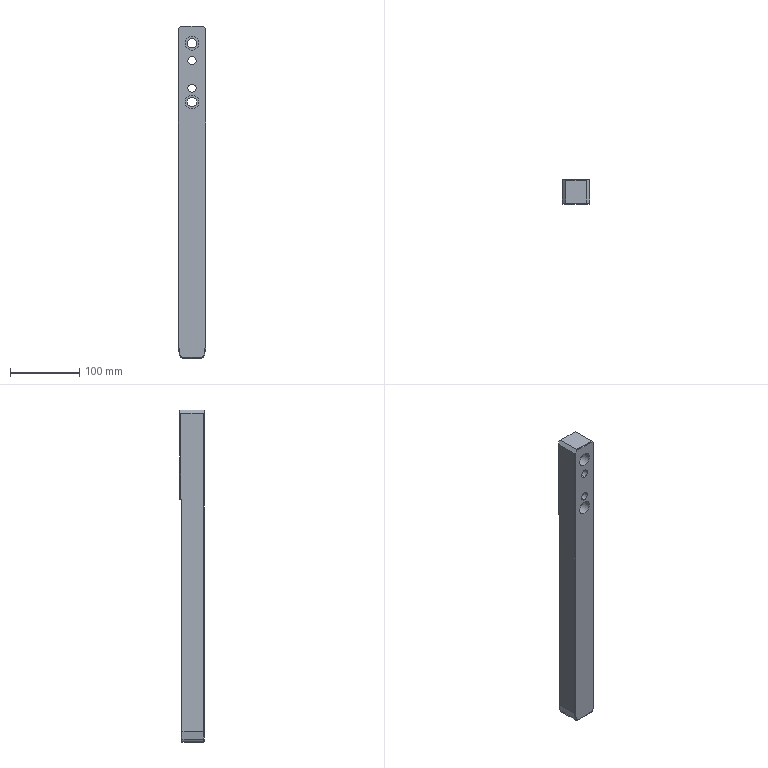Part | Creo | 1 solid | 46 faces | box 40 x 35 x 480 mm | volume 618107 mm3 | plane 28 | cylinder 14 | cone 4 | commonest cylinder face diameters 12 x4 13.5 x4 20 x4 10 x2
STEP:
#1=CARTESIAN_POINT('',(175.,-339.005,24.));
#2=VERTEX_POINT('',#1);
#3=CARTESIAN_POINT('',(175.,-339.005,36.));
#4=VERTEX_POINT('',#3);
#5=CARTESIAN_POINT('',(175.,-339.005,30.));
#6=DIRECTION('',(0.,-1.,0.));
#7=DIRECTION('',(0.,0.,-1.));
#8=AXIS2_PLACEMENT_3D('',#5,#6,#7);
#9=CIRCLE('',#8,6.);
#10=EDGE_CURVE('',#2,#4,#9,.T.);
#11=ORIENTED_EDGE('',*,*,#10,.T.);
#12=CARTESIAN_POINT('',(175.,-374.005,36.));
#13=VERTEX_POINT('',#12);
#14=CARTESIAN_POINT('',(175.,-374.005,36.));
#15=DIRECTION('',(0.,1.,0.));
#16=VECTOR('',#15,35.);
#17=LINE('',#14,#16);
#18=EDGE_CURVE('',#13,#4,#17,.T.);
#19=ORIENTED_EDGE('',*,*,#18,.F.);
#20=CARTESIAN_POINT('',(175.,-374.005,24.));
#21=VERTEX_POINT('',#20);
#22=CARTESIAN_POINT('',(175.,-374.005,30.));
#23=DIRECTION('',(0.,1.,0.));
#24=DIRECTION('',(0.,0.,1.));
#25=AXIS2_PLACEMENT_3D('',#22,#23,#24);
#26=CIRCLE('',#25,6.);
#27=EDGE_CURVE('',#13,#21,#26,.T.);
#28=ORIENTED_EDGE('',*,*,#27,.T.);
#29=CARTESIAN_POINT('',(175.,-374.005,24.));
#30=DIRECTION('',(0.,1.,0.));
#31=VECTOR('',#30,35.);
#32=LINE('',#29,#31);
#33=EDGE_CURVE('',#21,#2,#32,.T.);
#34=ORIENTED_EDGE('',*,*,#33,.T.);
#35=EDGE_LOOP('',(#11,#19,#28,#34));
#36=FACE_OUTER_BOUND('',#35,.F.);
#37=CARTESIAN_POINT('',(175.,-376.714,30.));
#38=DIRECTION('',(0.,1.,0.));
#39=DIRECTION('',(0.,0.,1.));
#40=AXIS2_PLACEMENT_3D('',#37,#38,#39);
#41=CYLINDRICAL_SURFACE('',#40,6.);
#42=ADVANCED_FACE('',(#36),#41,.F.);
#43=CARTESIAN_POINT('',(191.,-339.005,119.));
#44=VERTEX_POINT('',#43);
#45=CARTESIAN_POINT('',(159.,-339.005,119.));
#46=VERTEX_POINT('',#45);
#47=CARTESIAN_POINT('',(191.,-339.005,119.));
#48=DIRECTION('',(-1.,0.,0.));
#49=VECTOR('',#48,32.);
#50=LINE('',#47,#49);
#51=EDGE_CURVE('',#44,#46,#50,.T.);
#52=ORIENTED_EDGE('',*,*,#51,.T.);
#53=CARTESIAN_POINT('',(156.,-339.005,116.));
#54=VERTEX_POINT('',#53);
#55=CARTESIAN_POINT('',(156.,-339.005,116.));
#56=DIRECTION('',(0.7071,0.,0.7071));
#57=VECTOR('',#56,4.243);
#58=LINE('',#55,#57);
#59=EDGE_CURVE('',#54,#46,#58,.T.);
#60=ORIENTED_EDGE('',*,*,#59,.F.);
#61=CARTESIAN_POINT('',(156.,-339.005,-9.));
#62=VERTEX_POINT('',#61);
#63=CARTESIAN_POINT('',(156.,-339.005,116.));
#64=DIRECTION('',(0.,0.,-1.));
#65=VECTOR('',#64,125.);
#66=LINE('',#63,#65);
#67=EDGE_CURVE('',#54,#62,#66,.T.);
#68=ORIENTED_EDGE('',*,*,#67,.T.);
#69=CARTESIAN_POINT('',(194.,-339.005,-9.));
#70=VERTEX_POINT('',#69);
#71=CARTESIAN_POINT('',(194.,-339.005,-9.));
#72=DIRECTION('',(-1.,0.,0.));
#73=VECTOR('',#72,38.);
#74=LINE('',#71,#73);
#75=EDGE_CURVE('',#70,#62,#74,.T.);
#76=ORIENTED_EDGE('',*,*,#75,.F.);
#77=CARTESIAN_POINT('',(194.,-339.005,116.));
#78=VERTEX_POINT('',#77);
#79=CARTESIAN_POINT('',(194.,-339.005,-9.));
#80=DIRECTION('',(0.,0.,1.));
#81=VECTOR('',#80,125.);
#82=LINE('',#79,#81);
#83=EDGE_CURVE('',#70,#78,#82,.T.);
#84=ORIENTED_EDGE('',*,*,#83,.T.);
#85=CARTESIAN_POINT('',(191.,-339.005,119.));
#86=DIRECTION('',(0.7071,0.,-0.7071));
#87=VECTOR('',#86,4.243);
#88=LINE('',#85,#87);
#89=EDGE_CURVE('',#44,#78,#88,.T.);
#90=ORIENTED_EDGE('',*,*,#89,.F.);
#91=EDGE_LOOP('',(#52,#60,#68,#76,#84,#90));
#92=FACE_OUTER_BOUND('',#91,.F.);
#93=CARTESIAN_POINT('',(175.,-339.005,76.));
#94=VERTEX_POINT('',#93);
#95=CARTESIAN_POINT('',(175.,-339.005,64.));
#96=VERTEX_POINT('',#95);
#97=CARTESIAN_POINT('',(175.,-339.005,70.));
#98=DIRECTION('',(0.,-1.,0.));
#99=DIRECTION('',(0.,0.,1.));
#100=AXIS2_PLACEMENT_3D('',#97,#98,#99);
#101=CIRCLE('',#100,6.);
#102=EDGE_CURVE('',#94,#96,#101,.T.);
#103=ORIENTED_EDGE('',*,*,#102,.F.);
#104=CARTESIAN_POINT('',(175.,-339.005,70.));
#105=DIRECTION('',(0.,-1.,0.));
#106=DIRECTION('',(0.,0.,-1.));
#107=AXIS2_PLACEMENT_3D('',#104,#105,#106);
#108=CIRCLE('',#107,6.);
#109=EDGE_CURVE('',#96,#94,#108,.T.);
#110=ORIENTED_EDGE('',*,*,#109,.F.);
#111=EDGE_LOOP('',(#103,#110));
#112=FACE_BOUND('',#111,.F.);
#113=CARTESIAN_POINT('',(168.25,-339.005,10.));
#114=VERTEX_POINT('',#113);
#115=CARTESIAN_POINT('',(181.75,-339.005,10.));
#116=VERTEX_POINT('',#115);
#117=CARTESIAN_POINT('',(175.,-339.005,10.));
#118=DIRECTION('',(0.,-1.,0.));
#119=DIRECTION('',(-1.,0.,0.));
#120=AXIS2_PLACEMENT_3D('',#117,#118,#119);
#121=CIRCLE('',#120,6.75);
#122=EDGE_CURVE('',#114,#116,#121,.T.);
#123=ORIENTED_EDGE('',*,*,#122,.F.);
#124=CARTESIAN_POINT('',(175.,-339.005,10.));
#125=DIRECTION('',(0.,-1.,0.));
#126=DIRECTION('',(1.,0.,0.));
#127=AXIS2_PLACEMENT_3D('',#124,#125,#126);
#128=CIRCLE('',#127,6.75);
#129=EDGE_CURVE('',#116,#114,#128,.T.);
#130=ORIENTED_EDGE('',*,*,#129,.F.);
#131=EDGE_LOOP('',(#123,#130));
#132=FACE_BOUND('',#131,.F.);
#133=CARTESIAN_POINT('',(168.25,-339.005,95.));
#134=VERTEX_POINT('',#133);
#135=CARTESIAN_POINT('',(181.75,-339.005,95.));
#136=VERTEX_POINT('',#135);
#137=CARTESIAN_POINT('',(175.,-339.005,95.));
#138=DIRECTION('',(0.,-1.,0.));
#139=DIRECTION('',(-1.,0.,0.));
#140=AXIS2_PLACEMENT_3D('',#137,#138,#139);
#141=CIRCLE('',#140,6.75);
#142=EDGE_CURVE('',#134,#136,#141,.T.);
#143=ORIENTED_EDGE('',*,*,#142,.F.);
#144=CARTESIAN_POINT('',(175.,-339.005,95.));
#145=DIRECTION('',(0.,-1.,0.));
#146=DIRECTION('',(1.,0.,0.));
#147=AXIS2_PLACEMENT_3D('',#144,#145,#146);
#148=CIRCLE('',#147,6.75);
#149=EDGE_CURVE('',#136,#134,#148,.T.);
#150=ORIENTED_EDGE('',*,*,#149,.F.);
#151=EDGE_LOOP('',(#143,#150));
#152=FACE_BOUND('',#151,.F.);
#153=CARTESIAN_POINT('',(175.,-339.005,30.));
#154=DIRECTION('',(0.,-1.,0.));
#155=DIRECTION('',(0.,0.,1.));
#156=AXIS2_PLACEMENT_3D('',#153,#154,#155);
#157=CIRCLE('',#156,6.);
#158=EDGE_CURVE('',#4,#2,#157,.T.);
#159=ORIENTED_EDGE('',*,*,#158,.F.);
#160=ORIENTED_EDGE('',*,*,#10,.F.);
#161=EDGE_LOOP('',(#159,#160));
#162=FACE_BOUND('',#161,.F.);
#163=CARTESIAN_POINT('',(175.,-339.005,-30.));
#164=DIRECTION('',(0.,-1.,0.));
#165=DIRECTION('',(1.,0.,0.));
#166=AXIS2_PLACEMENT_3D('',#163,#164,#165);
#167=PLANE('',#166);
#168=ADVANCED_FACE('',(#92,#112,#132,#152,#162),#167,.F.);
#169=ORIENTED_EDGE('',*,*,#158,.T.);
#170=ORIENTED_EDGE('',*,*,#33,.F.);
#171=CARTESIAN_POINT('',(175.,-374.005,30.));
#172=DIRECTION('',(0.,1.,0.));
#173=DIRECTION('',(0.,0.,-1.));
#174=AXIS2_PLACEMENT_3D('',#171,#172,#173);
#175=CIRCLE('',#174,6.);
#176=EDGE_CURVE('',#21,#13,#175,.T.);
#177=ORIENTED_EDGE('',*,*,#176,.T.);
#178=ORIENTED_EDGE('',*,*,#18,.T.);
#179=EDGE_LOOP('',(#169,#170,#177,#178));
#180=FACE_OUTER_BOUND('',#179,.F.);
#181=CARTESIAN_POINT('',(175.,-376.714,30.));
#182=DIRECTION('',(0.,1.,0.));
#183=DIRECTION('',(0.,0.,1.));
#184=AXIS2_PLACEMENT_3D('',#181,#182,#183);
#185=CYLINDRICAL_SURFACE('',#184,6.);
#186=ADVANCED_FACE('',(#180),#185,.F.);
#187=CARTESIAN_POINT('',(194.,-374.005,116.));
#188=VERTEX_POINT('',#187);
#189=CARTESIAN_POINT('',(194.,-374.005,-344.913));
#190=VERTEX_POINT('',#189);
#191=CARTESIAN_POINT('',(194.,-374.005,116.));
#192=DIRECTION('',(0.,0.,-1.));
#193=VECTOR('',#192,460.913);
#194=LINE('',#191,#193);
#195=EDGE_CURVE('',#188,#190,#194,.T.);
#196=ORIENTED_EDGE('',*,*,#195,.T.);
#197=CARTESIAN_POINT('',(192.099,-374.005,-355.695));
#198=VERTEX_POINT('',#197);
#199=CARTESIAN_POINT('',(192.099,-374.005,-355.695));
#200=DIRECTION('',(0.1736,0.,0.9848));
#201=VECTOR('',#200,10.948);
#202=LINE('',#199,#201);
#203=EDGE_CURVE('',#198,#190,#202,.T.);
#204=ORIENTED_EDGE('',*,*,#203,.F.);
#205=CARTESIAN_POINT('',(188.16,-374.005,-359.));
#206=VERTEX_POINT('',#205);
#207=CARTESIAN_POINT('',(188.16,-374.005,-355.));
#208=DIRECTION('',(0.,-1.,0.));
#209=DIRECTION('',(0.,0.,-1.));
#210=AXIS2_PLACEMENT_3D('',#207,#208,#209);
#211=CIRCLE('',#210,4.);
#212=EDGE_CURVE('',#206,#198,#211,.T.);
#213=ORIENTED_EDGE('',*,*,#212,.F.);
#214=CARTESIAN_POINT('',(161.84,-374.005,-359.));
#215=VERTEX_POINT('',#214);
#216=CARTESIAN_POINT('',(188.16,-374.005,-359.));
#217=DIRECTION('',(-1.,0.,0.));
#218=VECTOR('',#217,26.319);
#219=LINE('',#216,#218);
#220=EDGE_CURVE('',#206,#215,#219,.T.);
#221=ORIENTED_EDGE('',*,*,#220,.T.);
#222=CARTESIAN_POINT('',(157.901,-374.005,-355.695));
#223=VERTEX_POINT('',#222);
#224=CARTESIAN_POINT('',(161.84,-374.005,-355.));
#225=DIRECTION('',(0.,-1.,0.));
#226=DIRECTION('',(-0.9848,0.,-0.1736));
#227=AXIS2_PLACEMENT_3D('',#224,#225,#226);
#228=CIRCLE('',#227,4.);
#229=EDGE_CURVE('',#223,#215,#228,.T.);
#230=ORIENTED_EDGE('',*,*,#229,.F.);
#231=CARTESIAN_POINT('',(156.,-374.005,-344.913));
#232=VERTEX_POINT('',#231);
#233=CARTESIAN_POINT('',(156.,-374.005,-344.913));
#234=DIRECTION('',(0.1736,0.,-0.9848));
#235=VECTOR('',#234,10.948);
#236=LINE('',#233,#235);
#237=EDGE_CURVE('',#232,#223,#236,.T.);
#238=ORIENTED_EDGE('',*,*,#237,.F.);
#239=CARTESIAN_POINT('',(156.,-374.005,116.));
#240=VERTEX_POINT('',#239);
#241=CARTESIAN_POINT('',(156.,-374.005,-344.913));
#242=DIRECTION('',(0.,0.,1.));
#243=VECTOR('',#242,460.913);
#244=LINE('',#241,#243);
#245=EDGE_CURVE('',#232,#240,#244,.T.);
#246=ORIENTED_EDGE('',*,*,#245,.T.);
#247=CARTESIAN_POINT('',(159.,-374.005,119.));
#248=VERTEX_POINT('',#247);
#249=CARTESIAN_POINT('',(159.,-374.005,119.));
#250=DIRECTION('',(-0.7071,0.,-0.7071));
#251=VECTOR('',#250,4.243);
#252=LINE('',#249,#251);
#253=EDGE_CURVE('',#248,#240,#252,.T.);
#254=ORIENTED_EDGE('',*,*,#253,.F.);
#255=CARTESIAN_POINT('',(191.,-374.005,119.));
#256=VERTEX_POINT('',#255);
#257=CARTESIAN_POINT('',(159.,-374.005,119.));
#258=DIRECTION('',(1.,0.,0.));
#259=VECTOR('',#258,32.);
#260=LINE('',#257,#259);
#261=EDGE_CURVE('',#248,#256,#260,.T.);
#262=ORIENTED_EDGE('',*,*,#261,.T.);
#263=CARTESIAN_POINT('',(194.,-374.005,116.));
#264=DIRECTION('',(-0.7071,0.,0.7071));
#265=VECTOR('',#264,4.243);
#266=LINE('',#263,#265);
#267=EDGE_CURVE('',#188,#256,#266,.T.);
#268=ORIENTED_EDGE('',*,*,#267,.F.);
#269=EDGE_LOOP('',(#196,#204,#213,#221,#230,#238,#246,#254,#262,#268));
#270=FACE_OUTER_BOUND('',#269,.F.);
#271=CARTESIAN_POINT('',(175.,-374.005,76.));
#272=VERTEX_POINT('',#271);
#273=CARTESIAN_POINT('',(175.,-374.005,64.));
#274=VERTEX_POINT('',#273);
#275=CARTESIAN_POINT('',(175.,-374.005,70.));
#276=DIRECTION('',(0.,1.,0.));
#277=DIRECTION('',(0.,0.,1.));
#278=AXIS2_PLACEMENT_3D('',#275,#276,#277);
#279=CIRCLE('',#278,6.);
#280=EDGE_CURVE('',#272,#274,#279,.T.);
#281=ORIENTED_EDGE('',*,*,#280,.F.);
#282=CARTESIAN_POINT('',(175.,-374.005,70.));
#283=DIRECTION('',(0.,1.,0.));
#284=DIRECTION('',(0.,0.,-1.));
#285=AXIS2_PLACEMENT_3D('',#282,#283,#284);
#286=CIRCLE('',#285,6.);
#287=EDGE_CURVE('',#274,#272,#286,.T.);
#288=ORIENTED_EDGE('',*,*,#287,.F.);
#289=EDGE_LOOP('',(#281,#288));
#290=FACE_BOUND('',#289,.F.);
#291=CARTESIAN_POINT('',(165.,-374.005,10.));
#292=VERTEX_POINT('',#291);
#293=CARTESIAN_POINT('',(185.,-374.005,10.));
#294=VERTEX_POINT('',#293);
#295=CARTESIAN_POINT('',(175.,-374.005,10.));
#296=DIRECTION('',(0.,1.,0.));
#297=DIRECTION('',(-1.,0.,0.));
#298=AXIS2_PLACEMENT_3D('',#295,#296,#297);
#299=CIRCLE('',#298,10.);
#300=EDGE_CURVE('',#292,#294,#299,.T.);
#301=ORIENTED_EDGE('',*,*,#300,.F.);
#302=CARTESIAN_POINT('',(175.,-374.005,10.));
#303=DIRECTION('',(0.,1.,0.));
#304=DIRECTION('',(1.,0.,0.));
#305=AXIS2_PLACEMENT_3D('',#302,#303,#304);
#306=CIRCLE('',#305,10.);
#307=EDGE_CURVE('',#294,#292,#306,.T.);
#308=ORIENTED_EDGE('',*,*,#307,.F.);
#309=EDGE_LOOP('',(#301,#308));
#310=FACE_BOUND('',#309,.F.);
#311=CARTESIAN_POINT('',(165.,-374.005,95.));
#312=VERTEX_POINT('',#311);
#313=CARTESIAN_POINT('',(185.,-374.005,95.));
#314=VERTEX_POINT('',#313);
#315=CARTESIAN_POINT('',(175.,-374.005,95.));
#316=DIRECTION('',(0.,1.,0.));
#317=DIRECTION('',(-1.,0.,0.));
#318=AXIS2_PLACEMENT_3D('',#315,#316,#317);
#319=CIRCLE('',#318,10.);
#320=EDGE_CURVE('',#312,#314,#319,.T.);
#321=ORIENTED_EDGE('',*,*,#320,.F.);
#322=CARTESIAN_POINT('',(175.,-374.005,95.));
#323=DIRECTION('',(0.,1.,0.));
#324=DIRECTION('',(1.,0.,0.));
#325=AXIS2_PLACEMENT_3D('',#322,#323,#324);
#326=CIRCLE('',#325,10.);
#327=EDGE_CURVE('',#314,#312,#326,.T.);
#328=ORIENTED_EDGE('',*,*,#327,.F.);
#329=EDGE_LOOP('',(#321,#328));
#330=FACE_BOUND('',#329,.F.);
#331=ORIENTED_EDGE('',*,*,#27,.F.);
#332=ORIENTED_EDGE('',*,*,#176,.F.);
#333=EDGE_LOOP('',(#331,#332));
#334=FACE_BOUND('',#333,.F.);
#335=CARTESIAN_POINT('',(175.,-374.005,-30.));
#336=DIRECTION('',(0.,-1.,0.));
#337=DIRECTION('',(1.,0.,0.));
#338=AXIS2_PLACEMENT_3D('',#335,#336,#337);
#339=PLANE('',#338);
#340=ADVANCED_FACE('',(#270,#290,#310,#330,#334),#339,.T.);
#341=ORIENTED_EDGE('',*,*,#109,.T.);
#342=CARTESIAN_POINT('',(175.,-374.005,76.));
#343=DIRECTION('',(0.,1.,0.));
#344=VECTOR('',#343,35.);
#345=LINE('',#342,#344);
#346=EDGE_CURVE('',#272,#94,#345,.T.);
#347=ORIENTED_EDGE('',*,*,#346,.F.);
#348=ORIENTED_EDGE('',*,*,#280,.T.);
#349=CARTESIAN_POINT('',(175.,-374.005,64.));
#350=DIRECTION('',(0.,1.,0.));
#351=VECTOR('',#350,35.);
#352=LINE('',#349,#351);
#353=EDGE_CURVE('',#274,#96,#352,.T.);
#354=ORIENTED_EDGE('',*,*,#353,.T.);
#355=EDGE_LOOP('',(#341,#347,#348,#354));
#356=FACE_OUTER_BOUND('',#355,.F.);
#357=CARTESIAN_POINT('',(175.,-376.714,70.));
#358=DIRECTION('',(0.,1.,0.));
#359=DIRECTION('',(0.,0.,1.));
#360=AXIS2_PLACEMENT_3D('',#357,#358,#359);
#361=CYLINDRICAL_SURFACE('',#360,6.);
#362=ADVANCED_FACE('',(#356),#361,.F.);
#363=ORIENTED_EDGE('',*,*,#102,.T.);
#364=ORIENTED_EDGE('',*,*,#353,.F.);
#365=ORIENTED_EDGE('',*,*,#287,.T.);
#366=ORIENTED_EDGE('',*,*,#346,.T.);
#367=EDGE_LOOP('',(#363,#364,#365,#366));
#368=FACE_OUTER_BOUND('',#367,.F.);
#369=CARTESIAN_POINT('',(175.,-376.714,70.));
#370=DIRECTION('',(0.,1.,0.));
#371=DIRECTION('',(0.,0.,1.));
#372=AXIS2_PLACEMENT_3D('',#369,#370,#371);
#373=CYLINDRICAL_SURFACE('',#372,6.);
#374=ADVANCED_FACE('',(#368),#373,.F.);
#375=ORIENTED_EDGE('',*,*,#300,.T.);
#376=CARTESIAN_POINT('',(185.,-361.005,10.));
#377=VERTEX_POINT('',#376);
#378=CARTESIAN_POINT('',(185.,-374.005,10.));
#379=DIRECTION('',(0.,1.,0.));
#380=VECTOR('',#379,13.);
#381=LINE('',#378,#380);
#382=EDGE_CURVE('',#294,#377,#381,.T.);
#383=ORIENTED_EDGE('',*,*,#382,.T.);
#384=CARTESIAN_POINT('',(165.,-361.005,10.));
#385=VERTEX_POINT('',#384);
#386=CARTESIAN_POINT('',(175.,-361.005,10.));
#387=DIRECTION('',(0.,-1.,0.));
#388=DIRECTION('',(1.,0.,0.));
#389=AXIS2_PLACEMENT_3D('',#386,#387,#388);
#390=CIRCLE('',#389,10.);
#391=EDGE_CURVE('',#377,#385,#390,.T.);
#392=ORIENTED_EDGE('',*,*,#391,.T.);
#393=CARTESIAN_POINT('',(165.,-374.005,10.));
#394=DIRECTION('',(0.,1.,0.));
#395=VECTOR('',#394,13.);
#396=LINE('',#393,#395);
#397=EDGE_CURVE('',#292,#385,#396,.T.);
#398=ORIENTED_EDGE('',*,*,#397,.F.);
#399=EDGE_LOOP('',(#375,#383,#392,#398));
#400=FACE_OUTER_BOUND('',#399,.F.);
#401=CARTESIAN_POINT('',(175.,-374.655,10.));
#402=DIRECTION('',(0.,1.,0.));
#403=DIRECTION('',(-1.,0.,0.));
#404=AXIS2_PLACEMENT_3D('',#401,#402,#403);
#405=CYLINDRICAL_SURFACE('',#404,10.);
#406=ADVANCED_FACE('',(#400),#405,.F.);
#407=ORIENTED_EDGE('',*,*,#307,.T.);
#408=ORIENTED_EDGE('',*,*,#397,.T.);
#409=CARTESIAN_POINT('',(175.,-361.005,10.));
#410=DIRECTION('',(0.,-1.,0.));
#411=DIRECTION('',(-1.,0.,0.));
#412=AXIS2_PLACEMENT_3D('',#409,#410,#411);
#413=CIRCLE('',#412,10.);
#414=EDGE_CURVE('',#385,#377,#413,.T.);
#415=ORIENTED_EDGE('',*,*,#414,.T.);
#416=ORIENTED_EDGE('',*,*,#382,.F.);
#417=EDGE_LOOP('',(#407,#408,#415,#416));
#418=FACE_OUTER_BOUND('',#417,.F.);
#419=CARTESIAN_POINT('',(175.,-374.655,10.));
#420=DIRECTION('',(0.,1.,0.));
#421=DIRECTION('',(-1.,0.,0.));
#422=AXIS2_PLACEMENT_3D('',#419,#420,#421);
#423=CYLINDRICAL_SURFACE('',#422,10.);
#424=ADVANCED_FACE('',(#418),#423,.F.);
#425=ORIENTED_EDGE('',*,*,#414,.F.);
#426=ORIENTED_EDGE('',*,*,#391,.F.);
#427=EDGE_LOOP('',(#425,#426));
#428=FACE_OUTER_BOUND('',#427,.F.);
#429=CARTESIAN_POINT('',(168.25,-361.005,10.));
#430=VERTEX_POINT('',#429);
#431=CARTESIAN_POINT('',(181.75,-361.005,10.));
#432=VERTEX_POINT('',#431);
#433=CARTESIAN_POINT('',(175.,-361.005,10.));
#434=DIRECTION('',(0.,1.,0.));
#435=DIRECTION('',(-1.,0.,0.));
#436=AXIS2_PLACEMENT_3D('',#433,#434,#435);
#437=CIRCLE('',#436,6.75);
#438=EDGE_CURVE('',#430,#432,#437,.T.);
#439=ORIENTED_EDGE('',*,*,#438,.F.);
#440=CARTESIAN_POINT('',(175.,-361.005,10.));
#441=DIRECTION('',(0.,1.,0.));
#442=DIRECTION('',(1.,0.,0.));
#443=AXIS2_PLACEMENT_3D('',#440,#441,#442);
#444=CIRCLE('',#443,6.75);
#445=EDGE_CURVE('',#432,#430,#444,.T.);
#446=ORIENTED_EDGE('',*,*,#445,.F.);
#447=EDGE_LOOP('',(#439,#446));
#448=FACE_BOUND('',#447,.F.);
#449=CARTESIAN_POINT('',(175.,-361.005,10.));
#450=DIRECTION('',(0.,1.,0.));
#451=DIRECTION('',(-1.,0.,0.));
#452=AXIS2_PLACEMENT_3D('',#449,#450,#451);
#453=PLANE('',#452);
#454=ADVANCED_FACE('',(#428,#448),#453,.F.);
#455=ORIENTED_EDGE('',*,*,#438,.T.);
#456=CARTESIAN_POINT('',(181.75,-339.005,10.));
#457=DIRECTION('',(0.,-1.,0.));
#458=VECTOR('',#457,22.);
#459=LINE('',#456,#458);
#460=EDGE_CURVE('',#116,#432,#459,.T.);
#461=ORIENTED_EDGE('',*,*,#460,.F.);
#462=ORIENTED_EDGE('',*,*,#129,.T.);
#463=CARTESIAN_POINT('',(168.25,-339.005,10.));
#464=DIRECTION('',(0.,-1.,0.));
#465=VECTOR('',#464,22.);
#466=LINE('',#463,#465);
#467=EDGE_CURVE('',#114,#430,#466,.T.);
#468=ORIENTED_EDGE('',*,*,#467,.T.);
#469=EDGE_LOOP('',(#455,#461,#462,#468));
#470=FACE_OUTER_BOUND('',#469,.F.);
#471=CARTESIAN_POINT('',(175.,-361.005,10.));
#472=DIRECTION('',(0.,-1.,0.));
#473=DIRECTION('',(-1.,0.,0.));
#474=AXIS2_PLACEMENT_3D('',#471,#472,#473);
#475=CYLINDRICAL_SURFACE('',#474,6.75);
#476=ADVANCED_FACE('',(#470),#475,.F.);
#477=ORIENTED_EDGE('',*,*,#445,.T.);
#478=ORIENTED_EDGE('',*,*,#467,.F.);
#479=ORIENTED_EDGE('',*,*,#122,.T.);
#480=ORIENTED_EDGE('',*,*,#460,.T.);
#481=EDGE_LOOP('',(#477,#478,#479,#480));
#482=FACE_OUTER_BOUND('',#481,.F.);
#483=CARTESIAN_POINT('',(175.,-361.005,10.));
#484=DIRECTION('',(0.,-1.,0.));
#485=DIRECTION('',(-1.,0.,0.));
#486=AXIS2_PLACEMENT_3D('',#483,#484,#485);
#487=CYLINDRICAL_SURFACE('',#486,6.75);
#488=ADVANCED_FACE('',(#482),#487,.F.);
#489=ORIENTED_EDGE('',*,*,#320,.T.);
#490=CARTESIAN_POINT('',(185.,-361.005,95.));
#491=VERTEX_POINT('',#490);
#492=CARTESIAN_POINT('',(185.,-374.005,95.));
#493=DIRECTION('',(0.,1.,0.));
#494=VECTOR('',#493,13.);
#495=LINE('',#492,#494);
#496=EDGE_CURVE('',#314,#491,#495,.T.);
#497=ORIENTED_EDGE('',*,*,#496,.T.);
#498=CARTESIAN_POINT('',(165.,-361.005,95.));
#499=VERTEX_POINT('',#498);
#500=CARTESIAN_POINT('',(175.,-361.005,95.));
#501=DIRECTION('',(0.,-1.,0.));
#502=DIRECTION('',(1.,0.,0.));
#503=AXIS2_PLACEMENT_3D('',#500,#501,#502);
#504=CIRCLE('',#503,10.);
#505=EDGE_CURVE('',#491,#499,#504,.T.);
#506=ORIENTED_EDGE('',*,*,#505,.T.);
#507=CARTESIAN_POINT('',(165.,-374.005,95.));
#508=DIRECTION('',(0.,1.,0.));
#509=VECTOR('',#508,13.);
#510=LINE('',#507,#509);
#511=EDGE_CURVE('',#312,#499,#510,.T.);
#512=ORIENTED_EDGE('',*,*,#511,.F.);
#513=EDGE_LOOP('',(#489,#497,#506,#512));
#514=FACE_OUTER_BOUND('',#513,.F.);
#515=CARTESIAN_POINT('',(175.,-374.655,95.));
#516=DIRECTION('',(0.,1.,0.));
#517=DIRECTION('',(-1.,0.,0.));
#518=AXIS2_PLACEMENT_3D('',#515,#516,#517);
#519=CYLINDRICAL_SURFACE('',#518,10.);
#520=ADVANCED_FACE('',(#514),#519,.F.);
#521=ORIENTED_EDGE('',*,*,#327,.T.);
#522=ORIENTED_EDGE('',*,*,#511,.T.);
#523=CARTESIAN_POINT('',(175.,-361.005,95.));
#524=DIRECTION('',(0.,-1.,0.));
#525=DIRECTION('',(-1.,0.,0.));
#526=AXIS2_PLACEMENT_3D('',#523,#524,#525);
#527=CIRCLE('',#526,10.);
#528=EDGE_CURVE('',#499,#491,#527,.T.);
#529=ORIENTED_EDGE('',*,*,#528,.T.);
#530=ORIENTED_EDGE('',*,*,#496,.F.);
#531=EDGE_LOOP('',(#521,#522,#529,#530));
#532=FACE_OUTER_BOUND('',#531,.F.);
#533=CARTESIAN_POINT('',(175.,-374.655,95.));
#534=DIRECTION('',(0.,1.,0.));
#535=DIRECTION('',(-1.,0.,0.));
#536=AXIS2_PLACEMENT_3D('',#533,#534,#535);
#537=CYLINDRICAL_SURFACE('',#536,10.);
#538=ADVANCED_FACE('',(#532),#537,.F.);
#539=ORIENTED_EDGE('',*,*,#528,.F.);
#540=ORIENTED_EDGE('',*,*,#505,.F.);
#541=EDGE_LOOP('',(#539,#540));
#542=FACE_OUTER_BOUND('',#541,.F.);
#543=CARTESIAN_POINT('',(168.25,-361.005,95.));
#544=VERTEX_POINT('',#543);
#545=CARTESIAN_POINT('',(181.75,-361.005,95.));
#546=VERTEX_POINT('',#545);
#547=CARTESIAN_POINT('',(175.,-361.005,95.));
#548=DIRECTION('',(0.,1.,0.));
#549=DIRECTION('',(-1.,0.,0.));
#550=AXIS2_PLACEMENT_3D('',#547,#548,#549);
#551=CIRCLE('',#550,6.75);
#552=EDGE_CURVE('',#544,#546,#551,.T.);
#553=ORIENTED_EDGE('',*,*,#552,.F.);
#554=CARTESIAN_POINT('',(175.,-361.005,95.));
#555=DIRECTION('',(0.,1.,0.));
#556=DIRECTION('',(1.,0.,0.));
#557=AXIS2_PLACEMENT_3D('',#554,#555,#556);
#558=CIRCLE('',#557,6.75);
#559=EDGE_CURVE('',#546,#544,#558,.T.);
#560=ORIENTED_EDGE('',*,*,#559,.F.);
#561=EDGE_LOOP('',(#553,#560));
#562=FACE_BOUND('',#561,.F.);
#563=CARTESIAN_POINT('',(175.,-361.005,95.));
#564=DIRECTION('',(0.,1.,0.));
#565=DIRECTION('',(-1.,0.,0.));
#566=AXIS2_PLACEMENT_3D('',#563,#564,#565);
#567=PLANE('',#566);
#568=ADVANCED_FACE('',(#542,#562),#567,.F.);
#569=ORIENTED_EDGE('',*,*,#552,.T.);
#570=CARTESIAN_POINT('',(181.75,-339.005,95.));
#571=DIRECTION('',(0.,-1.,0.));
#572=VECTOR('',#571,22.);
#573=LINE('',#570,#572);
#574=EDGE_CURVE('',#136,#546,#573,.T.);
#575=ORIENTED_EDGE('',*,*,#574,.F.);
#576=ORIENTED_EDGE('',*,*,#149,.T.);
#577=CARTESIAN_POINT('',(168.25,-339.005,95.));
#578=DIRECTION('',(0.,-1.,0.));
#579=VECTOR('',#578,22.);
#580=LINE('',#577,#579);
#581=EDGE_CURVE('',#134,#544,#580,.T.);
#582=ORIENTED_EDGE('',*,*,#581,.T.);
#583=EDGE_LOOP('',(#569,#575,#576,#582));
#584=FACE_OUTER_BOUND('',#583,.F.);
#585=CARTESIAN_POINT('',(175.,-361.005,95.));
#586=DIRECTION('',(0.,-1.,0.));
#587=DIRECTION('',(-1.,0.,0.));
#588=AXIS2_PLACEMENT_3D('',#585,#586,#587);
#589=CYLINDRICAL_SURFACE('',#588,6.75);
#590=ADVANCED_FACE('',(#584),#589,.F.);
#591=ORIENTED_EDGE('',*,*,#559,.T.);
#592=ORIENTED_EDGE('',*,*,#581,.F.);
#593=ORIENTED_EDGE('',*,*,#142,.T.);
#594=ORIENTED_EDGE('',*,*,#574,.T.);
#595=EDGE_LOOP('',(#591,#592,#593,#594));
#596=FACE_OUTER_BOUND('',#595,.F.);
#597=CARTESIAN_POINT('',(175.,-361.005,95.));
#598=DIRECTION('',(0.,-1.,0.));
#599=DIRECTION('',(-1.,0.,0.));
#600=AXIS2_PLACEMENT_3D('',#597,#598,#599);
#601=CYLINDRICAL_SURFACE('',#600,6.75);
#602=ADVANCED_FACE('',(#596),#601,.F.);
#603=CARTESIAN_POINT('',(195.,-373.005,115.));
#604=VERTEX_POINT('',#603);
#605=CARTESIAN_POINT('',(195.,-373.005,-345.));
#606=VERTEX_POINT('',#605);
#607=CARTESIAN_POINT('',(195.,-373.005,115.));
#608=DIRECTION('',(0.,0.,-1.));
#609=VECTOR('',#608,460.);
#610=LINE('',#607,#609);
#611=EDGE_CURVE('',#604,#606,#610,.T.);
#612=ORIENTED_EDGE('',*,*,#611,.T.);
#613=CARTESIAN_POINT('',(194.,-374.005,-344.913));
#614=DIRECTION('',(0.7058,0.7058,-0.06175));
#615=VECTOR('',#614,1.417);
#616=LINE('',#613,#615);
#617=EDGE_CURVE('',#190,#606,#616,.T.);
#618=ORIENTED_EDGE('',*,*,#617,.F.);
#619=ORIENTED_EDGE('',*,*,#195,.F.);
#620=CARTESIAN_POINT('',(194.,-374.005,116.));
#621=DIRECTION('',(0.5774,0.5774,-0.5774));
#622=VECTOR('',#621,1.732);
#623=LINE('',#620,#622);
#624=EDGE_CURVE('',#188,#604,#623,.T.);
#625=ORIENTED_EDGE('',*,*,#624,.T.);
#626=EDGE_LOOP('',(#612,#618,#619,#625));
#627=FACE_OUTER_BOUND('',#626,.F.);
#628=CARTESIAN_POINT('',(194.5,-373.505,-147.5));
#629=DIRECTION('',(0.7071,-0.7071,0.));
#630=DIRECTION('',(0.7071,0.7071,0.));
#631=AXIS2_PLACEMENT_3D('',#628,#629,#630);
#632=PLANE('',#631);
#633=ADVANCED_FACE('',(#627),#632,.T.);
#634=CARTESIAN_POINT('',(195.,-340.005,-9.));
#635=VERTEX_POINT('',#634);
#636=CARTESIAN_POINT('',(195.,-340.005,115.));
#637=VERTEX_POINT('',#636);
#638=CARTESIAN_POINT('',(195.,-340.005,-9.));
#639=DIRECTION('',(0.,0.,1.));
#640=VECTOR('',#639,124.);
#641=LINE('',#638,#640);
#642=EDGE_CURVE('',#635,#637,#641,.T.);
#643=ORIENTED_EDGE('',*,*,#642,.F.);
#644=CARTESIAN_POINT('',(195.,-342.005,-9.));
#645=VERTEX_POINT('',#644);
#646=CARTESIAN_POINT('',(195.,-340.005,-9.));
#647=DIRECTION('',(0.,-1.,0.));
#648=VECTOR('',#647,2.);
#649=LINE('',#646,#648);
#650=EDGE_CURVE('',#635,#645,#649,.T.);
#651=ORIENTED_EDGE('',*,*,#650,.T.);
#652=CARTESIAN_POINT('',(195.,-342.005,-345.));
#653=VERTEX_POINT('',#652);
#654=CARTESIAN_POINT('',(195.,-342.005,-9.));
#655=DIRECTION('',(0.,0.,-1.));
#656=VECTOR('',#655,336.);
#657=LINE('',#654,#656);
#658=EDGE_CURVE('',#645,#653,#657,.T.);
#659=ORIENTED_EDGE('',*,*,#658,.T.);
#660=CARTESIAN_POINT('',(195.,-342.005,-345.));
#661=DIRECTION('',(0.,-1.,0.));
#662=VECTOR('',#661,31.);
#663=LINE('',#660,#662);
#664=EDGE_CURVE('',#653,#606,#663,.T.);
#665=ORIENTED_EDGE('',*,*,#664,.T.);
#666=ORIENTED_EDGE('',*,*,#611,.F.);
#667=CARTESIAN_POINT('',(195.,-373.005,115.));
#668=DIRECTION('',(0.,1.,0.));
#669=VECTOR('',#668,33.);
#670=LINE('',#667,#669);
#671=EDGE_CURVE('',#604,#637,#670,.T.);
#672=ORIENTED_EDGE('',*,*,#671,.T.);
#673=EDGE_LOOP('',(#643,#651,#659,#665,#666,#672));
#674=FACE_OUTER_BOUND('',#673,.F.);
#675=CARTESIAN_POINT('',(195.,-339.005,-415.));
#676=DIRECTION('',(1.,0.,0.));
#677=DIRECTION('',(0.,0.,1.));
#678=AXIS2_PLACEMENT_3D('',#675,#676,#677);
#679=PLANE('',#678);
#680=ADVANCED_FACE('',(#674),#679,.T.);
#681=ORIENTED_EDGE('',*,*,#83,.F.);
#682=CARTESIAN_POINT('',(194.,-339.005,-9.));
#683=DIRECTION('',(0.7071,-0.7071,0.));
#684=VECTOR('',#683,1.414);
#685=LINE('',#682,#684);
#686=EDGE_CURVE('',#70,#635,#685,.T.);
#687=ORIENTED_EDGE('',*,*,#686,.T.);
#688=ORIENTED_EDGE('',*,*,#642,.T.);
#689=CARTESIAN_POINT('',(195.,-340.005,115.));
#690=DIRECTION('',(-0.5774,0.5774,0.5774));
#691=VECTOR('',#690,1.732);
#692=LINE('',#689,#691);
#693=EDGE_CURVE('',#637,#78,#692,.T.);
#694=ORIENTED_EDGE('',*,*,#693,.T.);
#695=EDGE_LOOP('',(#681,#687,#688,#694));
#696=FACE_OUTER_BOUND('',#695,.F.);
#697=CARTESIAN_POINT('',(194.5,-339.505,45.));
#698=DIRECTION('',(0.7071,0.7071,0.));
#699=DIRECTION('',(0.7071,-0.7071,0.));
#700=AXIS2_PLACEMENT_3D('',#697,#698,#699);
#701=PLANE('',#700);
#702=ADVANCED_FACE('',(#696),#701,.T.);
#703=CARTESIAN_POINT('',(156.,-341.005,-9.));
#704=VERTEX_POINT('',#703);
#705=CARTESIAN_POINT('',(155.,-342.005,-9.));
#706=VERTEX_POINT('',#705);
#707=CARTESIAN_POINT('',(156.,-341.005,-9.));
#708=DIRECTION('',(-0.7071,-0.7071,0.));
#709=VECTOR('',#708,1.414);
#710=LINE('',#707,#709);
#711=EDGE_CURVE('',#704,#706,#710,.T.);
#712=ORIENTED_EDGE('',*,*,#711,.F.);
#713=CARTESIAN_POINT('',(194.,-341.005,-9.));
#714=VERTEX_POINT('',#713);
#715=CARTESIAN_POINT('',(156.,-341.005,-9.));
#716=DIRECTION('',(1.,0.,0.));
#717=VECTOR('',#716,38.);
#718=LINE('',#715,#717);
#719=EDGE_CURVE('',#704,#714,#718,.T.);
#720=ORIENTED_EDGE('',*,*,#719,.T.);
#721=CARTESIAN_POINT('',(195.,-342.005,-9.));
#722=DIRECTION('',(-0.7071,0.7071,0.));
#723=VECTOR('',#722,1.414);
#724=LINE('',#721,#723);
#725=EDGE_CURVE('',#645,#714,#724,.T.);
#726=ORIENTED_EDGE('',*,*,#725,.F.);
#727=ORIENTED_EDGE('',*,*,#650,.F.);
#728=ORIENTED_EDGE('',*,*,#686,.F.);
#729=ORIENTED_EDGE('',*,*,#75,.T.);
#730=CARTESIAN_POINT('',(155.,-340.005,-9.));
#731=VERTEX_POINT('',#730);
#732=CARTESIAN_POINT('',(155.,-340.005,-9.));
#733=DIRECTION('',(0.7071,0.7071,0.));
#734=VECTOR('',#733,1.414);
#735=LINE('',#732,#734);
#736=EDGE_CURVE('',#731,#62,#735,.T.);
#737=ORIENTED_EDGE('',*,*,#736,.F.);
#738=CARTESIAN_POINT('',(155.,-342.005,-9.));
#739=DIRECTION('',(0.,1.,0.));
#740=VECTOR('',#739,2.);
#741=LINE('',#738,#740);
#742=EDGE_CURVE('',#706,#731,#741,.T.);
#743=ORIENTED_EDGE('',*,*,#742,.F.);
#744=EDGE_LOOP('',(#712,#720,#726,#727,#728,#729,#737,#743));
#745=FACE_OUTER_BOUND('',#744,.F.);
#746=CARTESIAN_POINT('',(195.,-339.005,-9.));
#747=DIRECTION('',(0.,0.,1.));
#748=DIRECTION('',(0.,-1.,0.));
#749=AXIS2_PLACEMENT_3D('',#746,#747,#748);
#750=PLANE('',#749);
#751=ADVANCED_FACE('',(#745),#750,.F.);
#752=ORIENTED_EDGE('',*,*,#711,.T.);
#753=CARTESIAN_POINT('',(155.,-342.005,-345.));
#754=VERTEX_POINT('',#753);
#755=CARTESIAN_POINT('',(155.,-342.005,-345.));
#756=DIRECTION('',(0.,0.,1.));
#757=VECTOR('',#756,336.);
#758=LINE('',#755,#757);
#759=EDGE_CURVE('',#754,#706,#758,.T.);
#760=ORIENTED_EDGE('',*,*,#759,.F.);
#761=CARTESIAN_POINT('',(156.,-341.005,-344.913));
#762=VERTEX_POINT('',#761);
#763=CARTESIAN_POINT('',(155.,-342.005,-345.));
#764=DIRECTION('',(0.7058,0.7058,0.06175));
#765=VECTOR('',#764,1.417);
#766=LINE('',#763,#765);
#767=EDGE_CURVE('',#754,#762,#766,.T.);
#768=ORIENTED_EDGE('',*,*,#767,.T.);
#769=CARTESIAN_POINT('',(156.,-341.005,-344.913));
#770=DIRECTION('',(0.,0.,1.));
#771=VECTOR('',#770,335.913);
#772=LINE('',#769,#771);
#773=EDGE_CURVE('',#762,#704,#772,.T.);
#774=ORIENTED_EDGE('',*,*,#773,.T.);
#775=EDGE_LOOP('',(#752,#760,#768,#774));
#776=FACE_OUTER_BOUND('',#775,.F.);
#777=CARTESIAN_POINT('',(155.5,-341.505,-222.5));
#778=DIRECTION('',(-0.7071,0.7071,0.));
#779=DIRECTION('',(0.7071,0.7071,0.));
#780=AXIS2_PLACEMENT_3D('',#777,#778,#779);
#781=PLANE('',#780);
#782=ADVANCED_FACE('',(#776),#781,.T.);
#783=CARTESIAN_POINT('',(155.,-373.005,-345.));
#784=VERTEX_POINT('',#783);
#785=CARTESIAN_POINT('',(155.,-373.005,115.));
#786=VERTEX_POINT('',#785);
#787=CARTESIAN_POINT('',(155.,-373.005,-345.));
#788=DIRECTION('',(0.,0.,1.));
#789=VECTOR('',#788,460.);
#790=LINE('',#787,#789);
#791=EDGE_CURVE('',#784,#786,#790,.T.);
#792=ORIENTED_EDGE('',*,*,#791,.F.);
#793=CARTESIAN_POINT('',(155.,-342.005,-345.));
#794=DIRECTION('',(0.,-1.,0.));
#795=VECTOR('',#794,31.);
#796=LINE('',#793,#795);
#797=EDGE_CURVE('',#754,#784,#796,.T.);
#798=ORIENTED_EDGE('',*,*,#797,.F.);
#799=ORIENTED_EDGE('',*,*,#759,.T.);
#800=ORIENTED_EDGE('',*,*,#742,.T.);
#801=CARTESIAN_POINT('',(155.,-340.005,115.));
#802=VERTEX_POINT('',#801);
#803=CARTESIAN_POINT('',(155.,-340.005,115.));
#804=DIRECTION('',(0.,0.,-1.));
#805=VECTOR('',#804,124.);
#806=LINE('',#803,#805);
#807=EDGE_CURVE('',#802,#731,#806,.T.);
#808=ORIENTED_EDGE('',*,*,#807,.F.);
#809=CARTESIAN_POINT('',(155.,-340.005,115.));
#810=DIRECTION('',(0.,-1.,0.));
#811=VECTOR('',#810,33.);
#812=LINE('',#809,#811);
#813=EDGE_CURVE('',#802,#786,#812,.T.);
#814=ORIENTED_EDGE('',*,*,#813,.T.);
#815=EDGE_LOOP('',(#792,#798,#799,#800,#808,#814));
#816=FACE_OUTER_BOUND('',#815,.F.);
#817=CARTESIAN_POINT('',(155.,-339.005,120.));
#818=DIRECTION('',(-1.,0.,0.));
#819=DIRECTION('',(0.,0.,-1.));
#820=AXIS2_PLACEMENT_3D('',#817,#818,#819);
#821=PLANE('',#820);
#822=ADVANCED_FACE('',(#816),#821,.T.);
#823=ORIENTED_EDGE('',*,*,#245,.F.);
#824=CARTESIAN_POINT('',(156.,-374.005,-344.913));
#825=DIRECTION('',(-0.7058,0.7058,-0.06175));
#826=VECTOR('',#825,1.417);
#827=LINE('',#824,#826);
#828=EDGE_CURVE('',#232,#784,#827,.T.);
#829=ORIENTED_EDGE('',*,*,#828,.T.);
#830=ORIENTED_EDGE('',*,*,#791,.T.);
#831=CARTESIAN_POINT('',(155.,-373.005,115.));
#832=DIRECTION('',(0.5774,-0.5774,0.5774));
#833=VECTOR('',#832,1.732);
#834=LINE('',#831,#833);
#835=EDGE_CURVE('',#786,#240,#834,.T.);
#836=ORIENTED_EDGE('',*,*,#835,.T.);
#837=EDGE_LOOP('',(#823,#829,#830,#836));
#838=FACE_OUTER_BOUND('',#837,.F.);
#839=CARTESIAN_POINT('',(155.5,-373.505,-147.5));
#840=DIRECTION('',(-0.7071,-0.7071,0.));
#841=DIRECTION('',(-0.7071,0.7071,0.));
#842=AXIS2_PLACEMENT_3D('',#839,#840,#841);
#843=PLANE('',#842);
#844=ADVANCED_FACE('',(#838),#843,.T.);
#845=ORIENTED_EDGE('',*,*,#828,.F.);
#846=ORIENTED_EDGE('',*,*,#237,.T.);
#847=CARTESIAN_POINT('',(156.916,-373.005,-355.868));
#848=VERTEX_POINT('',#847);
#849=CARTESIAN_POINT('',(156.916,-373.005,-355.868));
#850=DIRECTION('',(0.6964,-0.7071,0.1228));
#851=VECTOR('',#850,1.414);
#852=LINE('',#849,#851);
#853=EDGE_CURVE('',#848,#223,#852,.T.);
#854=ORIENTED_EDGE('',*,*,#853,.F.);
#855=CARTESIAN_POINT('',(156.916,-373.005,-355.868));
#856=DIRECTION('',(-0.1736,0.,0.9848));
#857=VECTOR('',#856,11.036);
#858=LINE('',#855,#857);
#859=EDGE_CURVE('',#848,#784,#858,.T.);
#860=ORIENTED_EDGE('',*,*,#859,.T.);
#861=EDGE_LOOP('',(#845,#846,#854,#860));
#862=FACE_OUTER_BOUND('',#861,.F.);
#863=CARTESIAN_POINT('',(156.451,-373.505,-350.347));
#864=DIRECTION('',(-0.6964,-0.7071,-0.1228));
#865=DIRECTION('',(-0.6964,0.7071,-0.1228));
#866=AXIS2_PLACEMENT_3D('',#863,#864,#865);
#867=PLANE('',#866);
#868=ADVANCED_FACE('',(#862),#867,.T.);
#869=ORIENTED_EDGE('',*,*,#853,.T.);
#870=ORIENTED_EDGE('',*,*,#229,.T.);
#871=CARTESIAN_POINT('',(161.84,-373.005,-360.));
#872=VERTEX_POINT('',#871);
#873=CARTESIAN_POINT('',(161.84,-373.005,-360.));
#874=DIRECTION('',(0.,-0.7071,0.7071));
#875=VECTOR('',#874,1.414);
#876=LINE('',#873,#875);
#877=EDGE_CURVE('',#872,#215,#876,.T.);
#878=ORIENTED_EDGE('',*,*,#877,.F.);
#879=CARTESIAN_POINT('',(161.84,-373.005,-355.));
#880=DIRECTION('',(0.,-1.,0.));
#881=DIRECTION('',(-0.9848,0.,-0.1736));
#882=AXIS2_PLACEMENT_3D('',#879,#880,#881);
#883=CIRCLE('',#882,5.);
#884=EDGE_CURVE('',#848,#872,#883,.T.);
#885=ORIENTED_EDGE('',*,*,#884,.F.);
#886=EDGE_LOOP('',(#869,#870,#878,#885));
#887=FACE_OUTER_BOUND('',#886,.F.);
#888=CARTESIAN_POINT('',(161.84,-373.505,-355.));
#889=DIRECTION('',(0.,1.,0.));
#890=DIRECTION('',(0.,0.,-1.));
#891=AXIS2_PLACEMENT_3D('',#888,#889,#890);
#892=CONICAL_SURFACE('',#891,4.5,45.);
#893=ADVANCED_FACE('',(#887),#892,.T.);
#894=ORIENTED_EDGE('',*,*,#877,.T.);
#895=ORIENTED_EDGE('',*,*,#220,.F.);
#896=CARTESIAN_POINT('',(188.16,-373.005,-360.));
#897=VERTEX_POINT('',#896);
#898=CARTESIAN_POINT('',(188.16,-373.005,-360.));
#899=DIRECTION('',(0.000000002,-0.7071,0.7071));
#900=VECTOR('',#899,1.414);
#901=LINE('',#898,#900);
#902=EDGE_CURVE('',#897,#206,#901,.T.);
#903=ORIENTED_EDGE('',*,*,#902,.F.);
#904=CARTESIAN_POINT('',(188.16,-373.005,-360.));
#905=DIRECTION('',(-1.,0.,0.));
#906=VECTOR('',#905,26.319);
#907=LINE('',#904,#906);
#908=EDGE_CURVE('',#897,#872,#907,.T.);
#909=ORIENTED_EDGE('',*,*,#908,.T.);
#910=EDGE_LOOP('',(#894,#895,#903,#909));
#911=FACE_OUTER_BOUND('',#910,.F.);
#912=CARTESIAN_POINT('',(175.,-373.505,-359.5));
#913=DIRECTION('',(0.,-0.7071,-0.7071));
#914=DIRECTION('',(0.,0.7071,-0.7071));
#915=AXIS2_PLACEMENT_3D('',#912,#913,#914);
#916=PLANE('',#915);
#917=ADVANCED_FACE('',(#911),#916,.T.);
#918=ORIENTED_EDGE('',*,*,#902,.T.);
#919=ORIENTED_EDGE('',*,*,#212,.T.);
#920=CARTESIAN_POINT('',(193.084,-373.005,-355.868));
#921=VERTEX_POINT('',#920);
#922=CARTESIAN_POINT('',(193.084,-373.005,-355.868));
#923=DIRECTION('',(-0.6964,-0.7071,0.1228));
#924=VECTOR('',#923,1.414);
#925=LINE('',#922,#924);
#926=EDGE_CURVE('',#921,#198,#925,.T.);
#927=ORIENTED_EDGE('',*,*,#926,.F.);
#928=CARTESIAN_POINT('',(188.16,-373.005,-355.));
#929=DIRECTION('',(0.,-1.,0.));
#930=DIRECTION('',(0.,0.,-1.));
#931=AXIS2_PLACEMENT_3D('',#928,#929,#930);
#932=CIRCLE('',#931,5.);
#933=EDGE_CURVE('',#897,#921,#932,.T.);
#934=ORIENTED_EDGE('',*,*,#933,.F.);
#935=EDGE_LOOP('',(#918,#919,#927,#934));
#936=FACE_OUTER_BOUND('',#935,.F.);
#937=CARTESIAN_POINT('',(188.16,-373.505,-355.));
#938=DIRECTION('',(0.,1.,0.));
#939=DIRECTION('',(0.,0.,-1.));
#940=AXIS2_PLACEMENT_3D('',#937,#938,#939);
#941=CONICAL_SURFACE('',#940,4.5,45.);
#942=ADVANCED_FACE('',(#936),#941,.T.);
#943=ORIENTED_EDGE('',*,*,#617,.T.);
#944=CARTESIAN_POINT('',(195.,-373.005,-345.));
#945=DIRECTION('',(-0.1736,0.,-0.9848));
#946=VECTOR('',#945,11.036);
#947=LINE('',#944,#946);
#948=EDGE_CURVE('',#606,#921,#947,.T.);
#949=ORIENTED_EDGE('',*,*,#948,.T.);
#950=ORIENTED_EDGE('',*,*,#926,.T.);
#951=ORIENTED_EDGE('',*,*,#203,.T.);
#952=EDGE_LOOP('',(#943,#949,#950,#951));
#953=FACE_OUTER_BOUND('',#952,.F.);
#954=CARTESIAN_POINT('',(193.549,-373.505,-350.347));
#955=DIRECTION('',(0.6964,-0.7071,-0.1228));
#956=DIRECTION('',(0.6964,0.7071,-0.1228));
#957=AXIS2_PLACEMENT_3D('',#954,#955,#956);
#958=PLANE('',#957);
#959=ADVANCED_FACE('',(#953),#958,.T.);
#960=ORIENTED_EDGE('',*,*,#664,.F.);
#961=CARTESIAN_POINT('',(193.084,-342.005,-355.868));
#962=VERTEX_POINT('',#961);
#963=CARTESIAN_POINT('',(195.,-342.005,-345.));
#964=DIRECTION('',(-0.1736,0.,-0.9848));
#965=VECTOR('',#964,11.036);
#966=LINE('',#963,#965);
#967=EDGE_CURVE('',#653,#962,#966,.T.);
#968=ORIENTED_EDGE('',*,*,#967,.T.);
#969=CARTESIAN_POINT('',(193.084,-342.005,-355.868));
#970=DIRECTION('',(-0.000000001,-1.,-0.000000005));
#971=VECTOR('',#970,31.);
#972=LINE('',#969,#971);
#973=EDGE_CURVE('',#962,#921,#972,.T.);
#974=ORIENTED_EDGE('',*,*,#973,.T.);
#975=ORIENTED_EDGE('',*,*,#948,.F.);
#976=EDGE_LOOP('',(#960,#968,#974,#975));
#977=FACE_OUTER_BOUND('',#976,.F.);
#978=CARTESIAN_POINT('',(192.355,-339.005,-360.));
#979=DIRECTION('',(0.9848,0.,-0.1736));
#980=DIRECTION('',(0.1736,0.,0.9848));
#981=AXIS2_PLACEMENT_3D('',#978,#979,#980);
#982=PLANE('',#981);
#983=ADVANCED_FACE('',(#977),#982,.T.);
#984=CARTESIAN_POINT('',(194.,-341.005,-344.913));
#985=VERTEX_POINT('',#984);
#986=CARTESIAN_POINT('',(195.,-342.005,-345.));
#987=DIRECTION('',(-0.7058,0.7058,0.06175));
#988=VECTOR('',#987,1.417);
#989=LINE('',#986,#988);
#990=EDGE_CURVE('',#653,#985,#989,.T.);
#991=ORIENTED_EDGE('',*,*,#990,.T.);
#992=CARTESIAN_POINT('',(192.099,-341.005,-355.695));
#993=VERTEX_POINT('',#992);
#994=CARTESIAN_POINT('',(194.,-341.005,-344.913));
#995=DIRECTION('',(-0.1736,0.,-0.9848));
#996=VECTOR('',#995,10.948);
#997=LINE('',#994,#996);
#998=EDGE_CURVE('',#985,#993,#997,.T.);
#999=ORIENTED_EDGE('',*,*,#998,.T.);
#1000=CARTESIAN_POINT('',(192.099,-341.005,-355.695));
#1001=DIRECTION('',(0.6964,-0.7071,-0.1228));
#1002=VECTOR('',#1001,1.414);
#1003=LINE('',#1000,#1002);
#1004=EDGE_CURVE('',#993,#962,#1003,.T.);
#1005=ORIENTED_EDGE('',*,*,#1004,.T.);
#1006=ORIENTED_EDGE('',*,*,#967,.F.);
#1007=EDGE_LOOP('',(#991,#999,#1005,#1006));
#1008=FACE_OUTER_BOUND('',#1007,.F.);
#1009=CARTESIAN_POINT('',(193.549,-341.505,-350.347));
#1010=DIRECTION('',(0.6964,0.7071,-0.1228));
#1011=DIRECTION('',(-0.6964,0.7071,0.1228));
#1012=AXIS2_PLACEMENT_3D('',#1009,#1010,#1011);
#1013=PLANE('',#1012);
#1014=ADVANCED_FACE('',(#1008),#1013,.T.);
#1015=ORIENTED_EDGE('',*,*,#725,.T.);
#1016=CARTESIAN_POINT('',(194.,-341.005,-9.));
#1017=DIRECTION('',(0.,0.,-1.));
#1018=VECTOR('',#1017,335.913);
#1019=LINE('',#1016,#1018);
#1020=EDGE_CURVE('',#714,#985,#1019,.T.);
#1021=ORIENTED_EDGE('',*,*,#1020,.T.);
#1022=ORIENTED_EDGE('',*,*,#990,.F.);
#1023=ORIENTED_EDGE('',*,*,#658,.F.);
#1024=EDGE_LOOP('',(#1015,#1021,#1022,#1023));
#1025=FACE_OUTER_BOUND('',#1024,.F.);
#1026=CARTESIAN_POINT('',(194.5,-341.505,-222.5));
#1027=DIRECTION('',(0.7071,0.7071,0.));
#1028=DIRECTION('',(-0.7071,0.7071,0.));
#1029=AXIS2_PLACEMENT_3D('',#1026,#1027,#1028);
#1030=PLANE('',#1029);
#1031=ADVANCED_FACE('',(#1025),#1030,.T.);
#1032=ORIENTED_EDGE('',*,*,#998,.F.);
#1033=ORIENTED_EDGE('',*,*,#1020,.F.);
#1034=ORIENTED_EDGE('',*,*,#719,.F.);
#1035=ORIENTED_EDGE('',*,*,#773,.F.);
#1036=CARTESIAN_POINT('',(157.901,-341.005,-355.695));
#1037=VERTEX_POINT('',#1036);
#1038=CARTESIAN_POINT('',(157.901,-341.005,-355.695));
#1039=DIRECTION('',(-0.1736,0.,0.9848));
#1040=VECTOR('',#1039,10.948);
#1041=LINE('',#1038,#1040);
#1042=EDGE_CURVE('',#1037,#762,#1041,.T.);
#1043=ORIENTED_EDGE('',*,*,#1042,.F.);
#1044=CARTESIAN_POINT('',(161.84,-341.005,-359.));
#1045=VERTEX_POINT('',#1044);
#1046=CARTESIAN_POINT('',(161.84,-341.005,-355.));
#1047=DIRECTION('',(0.,1.,0.));
#1048=DIRECTION('',(0.,0.,-1.));
#1049=AXIS2_PLACEMENT_3D('',#1046,#1047,#1048);
#1050=CIRCLE('',#1049,4.);
#1051=EDGE_CURVE('',#1045,#1037,#1050,.T.);
#1052=ORIENTED_EDGE('',*,*,#1051,.F.);
#1053=CARTESIAN_POINT('',(188.16,-341.005,-359.));
#1054=VERTEX_POINT('',#1053);
#1055=CARTESIAN_POINT('',(188.16,-341.005,-359.));
#1056=DIRECTION('',(-1.,0.,0.));
#1057=VECTOR('',#1056,26.319);
#1058=LINE('',#1055,#1057);
#1059=EDGE_CURVE('',#1054,#1045,#1058,.T.);
#1060=ORIENTED_EDGE('',*,*,#1059,.F.);
#1061=CARTESIAN_POINT('',(188.16,-341.005,-355.));
#1062=DIRECTION('',(0.,1.,0.));
#1063=DIRECTION('',(0.9848,0.,-0.1736));
#1064=AXIS2_PLACEMENT_3D('',#1061,#1062,#1063);
#1065=CIRCLE('',#1064,4.);
#1066=EDGE_CURVE('',#993,#1054,#1065,.T.);
#1067=ORIENTED_EDGE('',*,*,#1066,.F.);
#1068=EDGE_LOOP('',(#1032,#1033,#1034,#1035,#1043,#1052,#1060,#1067));
#1069=FACE_OUTER_BOUND('',#1068,.F.);
#1070=CARTESIAN_POINT('',(195.,-341.005,-30.));
#1071=DIRECTION('',(0.,-1.,0.));
#1072=DIRECTION('',(0.,0.,-1.));
#1073=AXIS2_PLACEMENT_3D('',#1070,#1071,#1072);
#1074=PLANE('',#1073);
#1075=ADVANCED_FACE('',(#1069),#1074,.F.);
#1076=ORIENTED_EDGE('',*,*,#767,.F.);
#1077=CARTESIAN_POINT('',(156.916,-342.005,-355.868));
#1078=VERTEX_POINT('',#1077);
#1079=CARTESIAN_POINT('',(156.916,-342.005,-355.868));
#1080=DIRECTION('',(-0.1736,0.,0.9848));
#1081=VECTOR('',#1080,11.036);
#1082=LINE('',#1079,#1081);
#1083=EDGE_CURVE('',#1078,#754,#1082,.T.);
#1084=ORIENTED_EDGE('',*,*,#1083,.F.);
#1085=CARTESIAN_POINT('',(157.901,-341.005,-355.695));
#1086=DIRECTION('',(-0.6964,-0.7071,-0.1228));
#1087=VECTOR('',#1086,1.414);
#1088=LINE('',#1085,#1087);
#1089=EDGE_CURVE('',#1037,#1078,#1088,.T.);
#1090=ORIENTED_EDGE('',*,*,#1089,.F.);
#1091=ORIENTED_EDGE('',*,*,#1042,.T.);
#1092=EDGE_LOOP('',(#1076,#1084,#1090,#1091));
#1093=FACE_OUTER_BOUND('',#1092,.F.);
#1094=CARTESIAN_POINT('',(156.451,-341.505,-350.347));
#1095=DIRECTION('',(-0.6964,0.7071,-0.1228));
#1096=DIRECTION('',(0.6964,0.7071,0.1228));
#1097=AXIS2_PLACEMENT_3D('',#1094,#1095,#1096);
#1098=PLANE('',#1097);
#1099=ADVANCED_FACE('',(#1093),#1098,.T.);
#1100=CARTESIAN_POINT('',(156.916,-373.005,-355.868));
#1101=DIRECTION('',(0.000000002,1.,-0.000000013));
#1102=VECTOR('',#1101,31.);
#1103=LINE('',#1100,#1102);
#1104=EDGE_CURVE('',#848,#1078,#1103,.T.);
#1105=ORIENTED_EDGE('',*,*,#1104,.T.);
#1106=ORIENTED_EDGE('',*,*,#1083,.T.);
#1107=ORIENTED_EDGE('',*,*,#797,.T.);
#1108=ORIENTED_EDGE('',*,*,#859,.F.);
#1109=EDGE_LOOP('',(#1105,#1106,#1107,#1108));
#1110=FACE_OUTER_BOUND('',#1109,.F.);
#1111=CARTESIAN_POINT('',(155.,-339.005,-345.));
#1112=DIRECTION('',(-0.9848,0.,-0.1736));
#1113=DIRECTION('',(0.1736,0.,-0.9848));
#1114=AXIS2_PLACEMENT_3D('',#1111,#1112,#1113);
#1115=PLANE('',#1114);
#1116=ADVANCED_FACE('',(#1110),#1115,.T.);
#1117=CARTESIAN_POINT('',(161.84,-342.005,-360.));
#1118=VERTEX_POINT('',#1117);
#1119=CARTESIAN_POINT('',(161.84,-342.005,-360.));
#1120=DIRECTION('',(0.,-1.,0.));
#1121=VECTOR('',#1120,31.);
#1122=LINE('',#1119,#1121);
#1123=EDGE_CURVE('',#1118,#872,#1122,.T.);
#1124=ORIENTED_EDGE('',*,*,#1123,.F.);
#1125=CARTESIAN_POINT('',(161.84,-342.005,-355.));
#1126=DIRECTION('',(0.,1.,0.));
#1127=DIRECTION('',(0.,0.,-1.));
#1128=AXIS2_PLACEMENT_3D('',#1125,#1126,#1127);
#1129=CIRCLE('',#1128,5.);
#1130=EDGE_CURVE('',#1118,#1078,#1129,.T.);
#1131=ORIENTED_EDGE('',*,*,#1130,.T.);
#1132=ORIENTED_EDGE('',*,*,#1104,.F.);
#1133=ORIENTED_EDGE('',*,*,#884,.T.);
#1134=EDGE_LOOP('',(#1124,#1131,#1132,#1133));
#1135=FACE_OUTER_BOUND('',#1134,.F.);
#1136=CARTESIAN_POINT('',(161.84,-374.953,-355.));
#1137=DIRECTION('',(0.,1.,0.));
#1138=DIRECTION('',(0.,0.,-1.));
#1139=AXIS2_PLACEMENT_3D('',#1136,#1137,#1138);
#1140=CYLINDRICAL_SURFACE('',#1139,5.);
#1141=ADVANCED_FACE('',(#1135),#1140,.T.);
#1142=CARTESIAN_POINT('',(188.16,-342.005,-360.));
#1143=VERTEX_POINT('',#1142);
#1144=CARTESIAN_POINT('',(188.16,-373.005,-360.));
#1145=DIRECTION('',(-0.000000001,1.,0.));
#1146=VECTOR('',#1145,31.);
#1147=LINE('',#1144,#1146);
#1148=EDGE_CURVE('',#897,#1143,#1147,.T.);
#1149=ORIENTED_EDGE('',*,*,#1148,.T.);
#1150=CARTESIAN_POINT('',(188.16,-342.005,-360.));
#1151=DIRECTION('',(-1.,0.,0.));
#1152=VECTOR('',#1151,26.319);
#1153=LINE('',#1150,#1152);
#1154=EDGE_CURVE('',#1143,#1118,#1153,.T.);
#1155=ORIENTED_EDGE('',*,*,#1154,.T.);
#1156=ORIENTED_EDGE('',*,*,#1123,.T.);
#1157=ORIENTED_EDGE('',*,*,#908,.F.);
#1158=EDGE_LOOP('',(#1149,#1155,#1156,#1157));
#1159=FACE_OUTER_BOUND('',#1158,.F.);
#1160=CARTESIAN_POINT('',(157.645,-339.005,-360.));
#1161=DIRECTION('',(0.,0.,-1.));
#1162=DIRECTION('',(1.,0.,0.));
#1163=AXIS2_PLACEMENT_3D('',#1160,#1161,#1162);
#1164=PLANE('',#1163);
#1165=ADVANCED_FACE('',(#1159),#1164,.T.);
#1166=ORIENTED_EDGE('',*,*,#973,.F.);
#1167=CARTESIAN_POINT('',(188.16,-342.005,-355.));
#1168=DIRECTION('',(0.,1.,0.));
#1169=DIRECTION('',(0.9848,0.,-0.1736));
#1170=AXIS2_PLACEMENT_3D('',#1167,#1168,#1169);
#1171=CIRCLE('',#1170,5.);
#1172=EDGE_CURVE('',#962,#1143,#1171,.T.);
#1173=ORIENTED_EDGE('',*,*,#1172,.T.);
#1174=ORIENTED_EDGE('',*,*,#1148,.F.);
#1175=ORIENTED_EDGE('',*,*,#933,.T.);
#1176=EDGE_LOOP('',(#1166,#1173,#1174,#1175));
#1177=FACE_OUTER_BOUND('',#1176,.F.);
#1178=CARTESIAN_POINT('',(188.16,-374.953,-355.));
#1179=DIRECTION('',(0.,1.,0.));
#1180=DIRECTION('',(0.9848,0.,-0.1736));
#1181=AXIS2_PLACEMENT_3D('',#1178,#1179,#1180);
#1182=CYLINDRICAL_SURFACE('',#1181,5.);
#1183=ADVANCED_FACE('',(#1177),#1182,.T.);
#1184=CARTESIAN_POINT('',(188.16,-342.005,-360.));
#1185=DIRECTION('',(0.,0.7071,0.7071));
#1186=VECTOR('',#1185,1.414);
#1187=LINE('',#1184,#1186);
#1188=EDGE_CURVE('',#1143,#1054,#1187,.T.);
#1189=ORIENTED_EDGE('',*,*,#1188,.F.);
#1190=ORIENTED_EDGE('',*,*,#1172,.F.);
#1191=ORIENTED_EDGE('',*,*,#1004,.F.);
#1192=ORIENTED_EDGE('',*,*,#1066,.T.);
#1193=EDGE_LOOP('',(#1189,#1190,#1191,#1192));
#1194=FACE_OUTER_BOUND('',#1193,.F.);
#1195=CARTESIAN_POINT('',(188.16,-341.505,-355.));
#1196=DIRECTION('',(0.,-1.,0.));
#1197=DIRECTION('',(0.,0.,-1.));
#1198=AXIS2_PLACEMENT_3D('',#1195,#1196,#1197);
#1199=CONICAL_SURFACE('',#1198,4.5,45.);
#1200=ADVANCED_FACE('',(#1194),#1199,.T.);
#1201=CARTESIAN_POINT('',(161.84,-341.005,-359.));
#1202=DIRECTION('',(0.,-0.7071,-0.7071));
#1203=VECTOR('',#1202,1.414);
#1204=LINE('',#1201,#1203);
#1205=EDGE_CURVE('',#1045,#1118,#1204,.T.);
#1206=ORIENTED_EDGE('',*,*,#1205,.T.);
#1207=ORIENTED_EDGE('',*,*,#1154,.F.);
#1208=ORIENTED_EDGE('',*,*,#1188,.T.);
#1209=ORIENTED_EDGE('',*,*,#1059,.T.);
#1210=EDGE_LOOP('',(#1206,#1207,#1208,#1209));
#1211=FACE_OUTER_BOUND('',#1210,.F.);
#1212=CARTESIAN_POINT('',(175.,-341.505,-359.5));
#1213=DIRECTION('',(0.,0.7071,-0.7071));
#1214=DIRECTION('',(0.,0.7071,0.7071));
#1215=AXIS2_PLACEMENT_3D('',#1212,#1213,#1214);
#1216=PLANE('',#1215);
#1217=ADVANCED_FACE('',(#1211),#1216,.T.);
#1218=ORIENTED_EDGE('',*,*,#1089,.T.);
#1219=ORIENTED_EDGE('',*,*,#1130,.F.);
#1220=ORIENTED_EDGE('',*,*,#1205,.F.);
#1221=ORIENTED_EDGE('',*,*,#1051,.T.);
#1222=EDGE_LOOP('',(#1218,#1219,#1220,#1221));
#1223=FACE_OUTER_BOUND('',#1222,.F.);
#1224=CARTESIAN_POINT('',(161.84,-341.505,-355.));
#1225=DIRECTION('',(0.,-1.,0.));
#1226=DIRECTION('',(0.,0.,-1.));
#1227=AXIS2_PLACEMENT_3D('',#1224,#1225,#1226);
#1228=CONICAL_SURFACE('',#1227,4.5,45.);
#1229=ADVANCED_FACE('',(#1223),#1228,.T.);
#1230=CARTESIAN_POINT('',(156.,-339.005,116.));
#1231=DIRECTION('',(-0.5774,-0.5774,-0.5774));
#1232=VECTOR('',#1231,1.732);
#1233=LINE('',#1230,#1232);
#1234=EDGE_CURVE('',#54,#802,#1233,.T.);
#1235=ORIENTED_EDGE('',*,*,#1234,.F.);
#1236=ORIENTED_EDGE('',*,*,#59,.T.);
#1237=CARTESIAN_POINT('',(160.,-340.005,120.));
#1238=VERTEX_POINT('',#1237);
#1239=CARTESIAN_POINT('',(160.,-340.005,120.));
#1240=DIRECTION('',(-0.5774,0.5774,-0.5774));
#1241=VECTOR('',#1240,1.732);
#1242=LINE('',#1239,#1241);
#1243=EDGE_CURVE('',#1238,#46,#1242,.T.);
#1244=ORIENTED_EDGE('',*,*,#1243,.F.);
#1245=CARTESIAN_POINT('',(160.,-373.005,120.));
#1246=VERTEX_POINT('',#1245);
#1247=CARTESIAN_POINT('',(160.,-373.005,120.));
#1248=DIRECTION('',(0.,1.,0.));
#1249=VECTOR('',#1248,33.);
#1250=LINE('',#1247,#1249);
#1251=EDGE_CURVE('',#1246,#1238,#1250,.T.);
#1252=ORIENTED_EDGE('',*,*,#1251,.F.);
#1253=CARTESIAN_POINT('',(159.,-374.005,119.));
#1254=DIRECTION('',(0.5774,0.5774,0.5774));
#1255=VECTOR('',#1254,1.732);
#1256=LINE('',#1253,#1255);
#1257=EDGE_CURVE('',#248,#1246,#1256,.T.);
#1258=ORIENTED_EDGE('',*,*,#1257,.F.);
#1259=ORIENTED_EDGE('',*,*,#253,.T.);
#1260=ORIENTED_EDGE('',*,*,#835,.F.);
#1261=ORIENTED_EDGE('',*,*,#813,.F.);
#1262=EDGE_LOOP('',(#1235,#1236,#1244,#1252,#1258,#1259,#1260,#1261));
#1263=FACE_OUTER_BOUND('',#1262,.F.);
#1264=CARTESIAN_POINT('',(160.,-339.005,120.));
#1265=DIRECTION('',(0.7071,0.,-0.7071));
#1266=DIRECTION('',(0.,1.,0.));
#1267=AXIS2_PLACEMENT_3D('',#1264,#1265,#1266);
#1268=PLANE('',#1267);
#1269=ADVANCED_FACE('',(#1263),#1268,.F.);
#1270=ORIENTED_EDGE('',*,*,#807,.T.);
#1271=ORIENTED_EDGE('',*,*,#736,.T.);
#1272=ORIENTED_EDGE('',*,*,#67,.F.);
#1273=ORIENTED_EDGE('',*,*,#1234,.T.);
#1274=EDGE_LOOP('',(#1270,#1271,#1272,#1273));
#1275=FACE_OUTER_BOUND('',#1274,.F.);
#1276=CARTESIAN_POINT('',(155.5,-339.505,45.));
#1277=DIRECTION('',(-0.7071,0.7071,0.));
#1278=DIRECTION('',(-0.7071,-0.7071,0.));
#1279=AXIS2_PLACEMENT_3D('',#1276,#1277,#1278);
#1280=PLANE('',#1279);
#1281=ADVANCED_FACE('',(#1275),#1280,.T.);
#1282=CARTESIAN_POINT('',(190.,-340.005,120.));
#1283=VERTEX_POINT('',#1282);
#1284=CARTESIAN_POINT('',(190.,-340.005,120.));
#1285=DIRECTION('',(-1.,0.,0.));
#1286=VECTOR('',#1285,30.);
#1287=LINE('',#1284,#1286);
#1288=EDGE_CURVE('',#1283,#1238,#1287,.T.);
#1289=ORIENTED_EDGE('',*,*,#1288,.T.);
#1290=ORIENTED_EDGE('',*,*,#1243,.T.);
#1291=ORIENTED_EDGE('',*,*,#51,.F.);
#1292=CARTESIAN_POINT('',(191.,-339.005,119.));
#1293=DIRECTION('',(-0.5774,-0.5774,0.5774));
#1294=VECTOR('',#1293,1.732);
#1295=LINE('',#1292,#1294);
#1296=EDGE_CURVE('',#44,#1283,#1295,.T.);
#1297=ORIENTED_EDGE('',*,*,#1296,.T.);
#1298=EDGE_LOOP('',(#1289,#1290,#1291,#1297));
#1299=FACE_OUTER_BOUND('',#1298,.F.);
#1300=CARTESIAN_POINT('',(175.,-339.505,119.5));
#1301=DIRECTION('',(0.,0.7071,0.7071));
#1302=DIRECTION('',(0.,-0.7071,0.7071));
#1303=AXIS2_PLACEMENT_3D('',#1300,#1301,#1302);
#1304=PLANE('',#1303);
#1305=ADVANCED_FACE('',(#1299),#1304,.T.);
#1306=CARTESIAN_POINT('',(190.,-373.005,120.));
#1307=VERTEX_POINT('',#1306);
#1308=CARTESIAN_POINT('',(160.,-373.005,120.));
#1309=DIRECTION('',(1.,0.,0.));
#1310=VECTOR('',#1309,30.);
#1311=LINE('',#1308,#1310);
#1312=EDGE_CURVE('',#1246,#1307,#1311,.T.);
#1313=ORIENTED_EDGE('',*,*,#1312,.F.);
#1314=ORIENTED_EDGE('',*,*,#1251,.T.);
#1315=ORIENTED_EDGE('',*,*,#1288,.F.);
#1316=CARTESIAN_POINT('',(190.,-340.005,120.));
#1317=DIRECTION('',(0.,-1.,0.));
#1318=VECTOR('',#1317,33.);
#1319=LINE('',#1316,#1318);
#1320=EDGE_CURVE('',#1283,#1307,#1319,.T.);
#1321=ORIENTED_EDGE('',*,*,#1320,.T.);
#1322=EDGE_LOOP('',(#1313,#1314,#1315,#1321));
#1323=FACE_OUTER_BOUND('',#1322,.F.);
#1324=CARTESIAN_POINT('',(195.,-339.005,120.));
#1325=DIRECTION('',(0.,0.,1.));
#1326=DIRECTION('',(-1.,0.,0.));
#1327=AXIS2_PLACEMENT_3D('',#1324,#1325,#1326);
#1328=PLANE('',#1327);
#1329=ADVANCED_FACE('',(#1323),#1328,.T.);
#1330=ORIENTED_EDGE('',*,*,#261,.F.);
#1331=ORIENTED_EDGE('',*,*,#1257,.T.);
#1332=ORIENTED_EDGE('',*,*,#1312,.T.);
#1333=CARTESIAN_POINT('',(190.,-373.005,120.));
#1334=DIRECTION('',(0.5774,-0.5774,-0.5774));
#1335=VECTOR('',#1334,1.732);
#1336=LINE('',#1333,#1335);
#1337=EDGE_CURVE('',#1307,#256,#1336,.T.);
#1338=ORIENTED_EDGE('',*,*,#1337,.T.);
#1339=EDGE_LOOP('',(#1330,#1331,#1332,#1338));
#1340=FACE_OUTER_BOUND('',#1339,.F.);
#1341=CARTESIAN_POINT('',(175.,-373.505,119.5));
#1342=DIRECTION('',(0.,-0.7071,0.7071));
#1343=DIRECTION('',(0.,0.7071,0.7071));
#1344=AXIS2_PLACEMENT_3D('',#1341,#1342,#1343);
#1345=PLANE('',#1344);
#1346=ADVANCED_FACE('',(#1340),#1345,.T.);
#1347=ORIENTED_EDGE('',*,*,#1296,.F.);
#1348=ORIENTED_EDGE('',*,*,#89,.T.);
#1349=ORIENTED_EDGE('',*,*,#693,.F.);
#1350=ORIENTED_EDGE('',*,*,#671,.F.);
#1351=ORIENTED_EDGE('',*,*,#624,.F.);
#1352=ORIENTED_EDGE('',*,*,#267,.T.);
#1353=ORIENTED_EDGE('',*,*,#1337,.F.);
#1354=ORIENTED_EDGE('',*,*,#1320,.F.);
#1355=EDGE_LOOP('',(#1347,#1348,#1349,#1350,#1351,#1352,#1353,#1354));
#1356=FACE_OUTER_BOUND('',#1355,.F.);
#1357=CARTESIAN_POINT('',(195.,-339.005,115.));
#1358=DIRECTION('',(-0.7071,0.,-0.7071));
#1359=DIRECTION('',(0.,1.,0.));
#1360=AXIS2_PLACEMENT_3D('',#1357,#1358,#1359);
#1361=PLANE('',#1360);
#1362=ADVANCED_FACE('',(#1356),#1361,.F.);
#1363=CLOSED_SHELL('',(#42,#168,#186,#340,#362,#374,#406,#424,#454,#476,#488,#520,#538,#568,#590,#602,#633,#680,#702,#751,#782,#822,#844,#868,#893,#917,#942,#959,#983,#1014,#1031,#1075,#1099,#1116,#1141,#1165,#1183,#1200,#1217,#1229,#1269,#1281,#1305,#1329,#1346,#1362));
#1364=MANIFOLD_SOLID_BREP('',#1363);
#1365=(LENGTH_UNIT()NAMED_UNIT(*)SI_UNIT(.MILLI.,.METRE.));
#1366=UNCERTAINTY_MEASURE_WITH_UNIT(LENGTH_MEASURE(0.04829),#1365,'','');
#1367=(NAMED_UNIT(*)PLANE_ANGLE_UNIT()SI_UNIT($,.RADIAN.));
#1368=PLANE_ANGLE_MEASURE_WITH_UNIT(PLANE_ANGLE_MEASURE(0.01745),#1367);
#1369=(CONVERSION_BASED_UNIT('DEGREE',#1368)NAMED_UNIT(*)PLANE_ANGLE_UNIT());
#1370=(NAMED_UNIT(*)SI_UNIT($,.STERADIAN.)SOLID_ANGLE_UNIT());
#1371=(GEOMETRIC_REPRESENTATION_CONTEXT(3)GLOBAL_UNCERTAINTY_ASSIGNED_CONTEXT((#1366))GLOBAL_UNIT_ASSIGNED_CONTEXT((#1365,#1369,#1370))REPRESENTATION_CONTEXT('',''));
#1372=ADVANCED_BREP_SHAPE_REPRESENTATION('',(#1364),#1371);